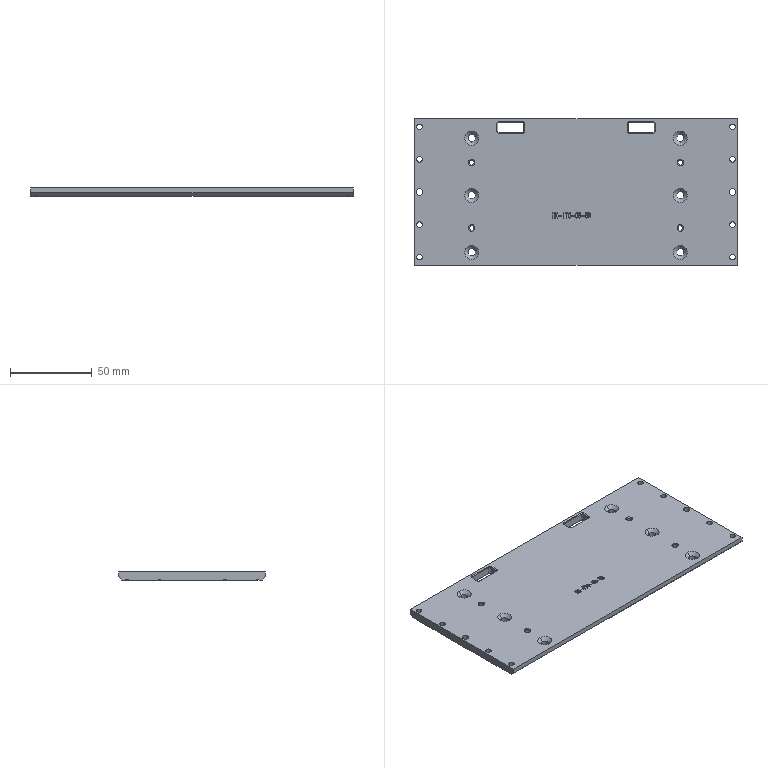NC program | NX | posted with a generic post | part box 198 x 90 x 5 mm
Lines 3242 to 4034 of 7160:
(ZLEVEL_PROFILE_COPY_1_COPY_COPY_COPY_1 , TOOL : D6A45)
N6422 T01 M6
N6424 G54
N6426 G17 G0 G90 X-98.522 Y18.565 S9500 M3
N6428 G43 Z30. H1
N6430 Z1.5
N6432 G94 G1 X-98.422 Y18.405 Z1.49 F1000.
N6434 X-98.29 Y18.203 Z1.477
N6436 X-97.857 Y17.759 Z1.445
N6438 X-97.339 Y17.416 Z1.412
N6440 X-96.76 Y17.19 Z1.38
N6442 X-96.147 Y17.093 Z1.347
N6444 X-95.527 Y17.128 Z1.315
N6446 X-94.929 Y17.293 Z1.282
N6448 X-94.379 Y17.582 Z1.25
N6450 X-94.002 Y17.882 Z1.224
N6452 X-93.599 Y18.354 Z1.192
N6454 X-93.304 Y18.901 Z1.159
N6456 X-93.132 Y19.497 Z1.127
N6458 X-93.091 Y20.117 Z1.094
N6460 X-93.182 Y20.731 Z1.062
N6462 X-93.401 Y21.312 Z1.029
N6464 X-93.738 Y21.833 Z0.997
N6466 X-94.071 Y22.181 Z0.971
N6468 X-94.578 Y22.54 Z0.939
N6470 X-95.149 Y22.784 Z0.906
N6472 X-95.758 Y22.901 Z0.874
N6474 X-96.379 Y22.886 Z0.841
N6476 X-96.982 Y22.74 Z0.809
N6478 X-97.541 Y22.469 Z0.776
N6480 X-98.03 Y22.086 Z0.744
N6482 X-98.188 Y21.904 Z0.731
N6484 X-98.237 Y21.848 Z0.727
N6486 X-98.619 Y21.317 Z0.693
N6488 X-98.657 Y21.245 Z0.689
N6490 X-98.76 Y21.024 Z0.676
N6492 X-98.918 Y20.378 Z0.641
N6494 X-98.927 Y19.713 Z0.606
N6496 X-98.788 Y19.062 Z0.571
N6498 X-98.692 Y18.838 Z0.558
N6500 X-98.422 Y18.405 Z0.532
N6502 X-98.29 Y18.203 Z0.519
N6504 X-97.857 Y17.759 Z0.486
N6506 X-97.339 Y17.416 Z0.454
N6508 X-96.76 Y17.19 Z0.421
N6510 X-96.147 Y17.093 Z0.389
N6512 X-95.527 Y17.128 Z0.356
N6514 X-94.929 Y17.293 Z0.324
N6516 X-94.379 Y17.582 Z0.291
N6518 X-94.002 Y17.882 Z0.266
N6520 X-93.599 Y18.354 Z0.233
N6522 X-93.304 Y18.901 Z0.201
N6524 X-93.132 Y19.497 Z0.168
N6526 X-93.091 Y20.117 Z0.136
N6528 X-93.182 Y20.731 Z0.103
N6530 X-93.401 Y21.312 Z0.071
N6532 X-93.738 Y21.833 Z0.038
N6534 X-94.071 Y22.181 Z0.013
N6536 X-94.578 Y22.54 Z-0.02
N6538 X-95.149 Y22.784 Z-0.052
N6540 X-95.758 Y22.901 Z-0.085
N6542 X-96.379 Y22.886 Z-0.117
N6544 X-96.982 Y22.74 Z-0.15
N6546 X-97.541 Y22.469 Z-0.182
N6548 X-98.03 Y22.086 Z-0.215
N6550 X-98.188 Y21.904 Z-0.227
N6552 X-98.237 Y21.848 Z-0.231
N6554 X-98.619 Y21.317 Z-0.266
N6556 X-98.657 Y21.245 Z-0.27
N6558 X-98.76 Y21.024 Z-0.283
N6560 X-98.918 Y20.378 Z-0.318
N6562 X-98.927 Y19.713 Z-0.352
N6564 X-98.788 Y19.062 Z-0.387
N6566 X-98.692 Y18.838 Z-0.4
N6568 X-98.422 Y18.405 F1300.
N6570 G3 X-98.188 Y21.904 R-2.901
N6572 G1 X-98.237 Y21.848
N6574 X-98.619 Y21.317
N6576 X-98.657 Y21.245
N6578 G3 X-98.692 Y18.838 R2.956
N6580 G1 X-98.624 Y18.722 Z-0.403
N6582 X-98.551 Y18.609 Z-0.406
N6584 X-98.413 Y18.411 Z-0.412
N6586 X-98.311 Y18.28 Z-0.416
N6588 X-98.207 Y18.149 Z-0.42
N6590 X-98.138 Y18.073 Z-0.422
N6592 X-97.983 Y17.922 Z-0.427
N6594 X-97.817 Y17.781 Z-0.432
N6596 X-97.642 Y17.655 Z-0.438
N6598 X-97.457 Y17.542 Z-0.443
N6600 X-97.266 Y17.444 Z-0.448
N6602 X-97.067 Y17.36 Z-0.453
N6604 X-96.864 Y17.292 Z-0.458
N6606 X-96.655 Y17.239 Z-0.463
N6608 X-96.445 Y17.202 Z-0.468
N6610 X-96.231 Y17.182 Z-0.473
N6612 X-96.019 Y17.177 Z-0.478
N6614 X-95.805 Y17.19 Z-0.483
N6616 X-95.595 Y17.216 Z-0.488
N6618 X-95.387 Y17.261 Z-0.493
N6620 X-95.183 Y17.318 Z-0.498
N6622 X-94.985 Y17.394 Z-0.503
N6624 X-94.793 Y17.48 Z-0.508
N6626 X-94.61 Y17.585 Z-0.513
N6628 X-94.433 Y17.698 Z-0.518
N6630 X-94.268 Y17.829 Z-0.523
N6632 X-94.163 Y17.924 Z-0.526
N6634 X-94.06 Y18.022 Z-0.53
N6636 X-93.969 Y18.121 Z-0.533
N6638 X-93.836 Y18.282 Z-0.538
N6640 X-93.717 Y18.454 Z-0.543
N6642 X-93.611 Y18.632 Z-0.548
N6644 X-93.519 Y18.819 Z-0.552
N6646 X-93.441 Y19.011 Z-0.557
N6648 X-93.379 Y19.209 Z-0.562
N6650 X-93.331 Y19.409 Z-0.567
N6652 X-93.3 Y19.613 Z-0.572
N6654 X-93.282 Y19.818 Z-0.577
N6656 X-93.281 Y20.024 Z-0.582
N6658 X-93.296 Y20.228 Z-0.586
N6660 X-93.326 Y20.431 Z-0.591
N6662 X-93.371 Y20.63 Z-0.596
N6664 X-93.43 Y20.826 Z-0.601
N6666 X-93.505 Y21.015 Z-0.606
N6668 X-93.592 Y21.199 Z-0.611
N6670 X-93.694 Y21.374 Z-0.615
N6672 X-93.807 Y21.542 Z-0.62
N6674 X-93.935 Y21.699 Z-0.625
N6676 X-94.071 Y21.848 Z-0.63
N6678 X-94.158 Y21.928 Z-0.632
N6680 X-94.245 Y22.007 Z-0.635
N6682 X-94.377 Y22.109 Z-0.639
N6684 X-94.544 Y22.22 Z-0.644
N6686 X-94.717 Y22.321 Z-0.649
N6688 X-94.899 Y22.405 Z-0.653
N6690 X-95.084 Y22.479 Z-0.658
N6692 X-95.276 Y22.534 Z-0.663
N6694 X-95.47 Y22.58 Z-0.667
N6696 X-95.666 Y22.605 Z-0.672
N6698 X-95.864 Y22.621 Z-0.677
N6700 X-96.062 Y22.616 Z-0.682
N6702 X-96.259 Y22.602 Z-0.686
N6704 X-96.453 Y22.567 Z-0.691
N6706 X-96.646 Y22.525 Z-0.695
N6708 X-96.831 Y22.461 Z-0.7
N6710 X-97.014 Y22.39 Z-0.705
N6712 X-97.188 Y22.299 Z-0.709
N6714 X-97.358 Y22.203 Z-0.714
N6716 X-97.514 Y22.087 Z-0.719
N6718 X-97.668 Y21.966 Z-0.723
N6720 X-97.805 Y21.828 Z-0.728
N6722 X-97.938 Y21.687 Z-0.732
N6724 X-97.98 Y21.636 Z-0.734
N6726 X-98.017 Y21.588 Z-0.735
N6728 X-98.052 Y21.539 Z-0.737
N6730 X-98.185 Y21.351 Z-0.742
N6732 X-98.311 Y21.151 Z-0.748
N6734 X-98.345 Y21.088 Z-0.749
N6736 X-98.408 Y20.924 Z-0.754
N6738 X-98.464 Y20.756 Z-0.758
N6740 X-98.522 Y20.473 Z-0.765
N6742 X-98.535 Y20.394 Z-0.766
N6744 X-98.547 Y20.216 Z-0.771
N6746 X-98.558 Y20.037 Z-0.775
N6748 X-98.529 Y19.682 Z-0.783
N6750 X-98.453 Y19.336 Z-0.792
N6752 X-98.396 Y19.169 Z-0.796
N6754 X-98.323 Y19.007 Z-0.8
N6756 X-98.231 Y18.848 Z-0.805
N6758 X-98.128 Y18.694 Z-0.81
N6760 X-97.9 Y18.407 Z-0.82
N6762 X-97.756 Y18.263 Z-0.826
N6764 X-97.605 Y18.126 Z-0.832
N6766 X-97.441 Y18.007 Z-0.837
N6768 X-97.27 Y17.898 Z-0.843
N6770 X-97.091 Y17.805 Z-0.848
N6772 X-96.903 Y17.729 Z-0.854
N6774 X-96.713 Y17.665 Z-0.86
N6776 X-96.516 Y17.622 Z-0.865
N6778 X-96.318 Y17.593 Z-0.871
N6780 X-96.118 Y17.581 Z-0.876
N6782 X-95.919 Y17.586 Z-0.882
N6784 X-95.721 Y17.606 Z-0.887
N6786 X-95.527 Y17.644 Z-0.893
N6788 X-95.334 Y17.693 Z-0.898
N6790 X-95.151 Y17.765 Z-0.904
N6792 X-94.968 Y17.841 Z-0.909
N6794 X-94.796 Y17.941 Z-0.915
N6796 X-94.635 Y18.05 Z-0.92
N6798 X-94.487 Y18.177 Z-0.926
N6800 X-94.343 Y18.31 Z-0.931
N6802 X-94.216 Y18.457 Z-0.936
N6804 X-94.097 Y18.611 Z-0.942
N6806 X-93.995 Y18.776 Z-0.947
N6808 X-93.904 Y18.947 Z-0.952
N6810 X-93.829 Y19.124 Z-0.958
N6812 X-93.77 Y19.308 Z-0.963
N6814 X-93.725 Y19.495 Z-0.969
N6816 X-93.697 Y19.685 Z-0.974
N6818 X-93.685 Y19.875 Z-0.979
N6820 X-93.687 Y20.067 Z-0.984
N6822 X-93.708 Y20.255 Z-0.99
N6824 X-93.739 Y20.443 Z-0.995
N6826 X-93.766 Y20.546 Z-0.998
N6828 X-93.795 Y20.649 Z-1.001
N6830 X-93.852 Y20.804 Z-1.005
N6832 X-93.934 Y20.974 Z-1.011
N6834 X-94.02 Y21.142 Z-1.016
N6836 X-94.124 Y21.292 Z-1.021
N6838 X-94.243 Y21.443 Z-1.026
N6840 X-94.375 Y21.575 Z-1.032
N6842 X-94.51 Y21.703 Z-1.037
N6844 X-94.66 Y21.813 Z-1.042
N6846 X-94.815 Y21.916 Z-1.047
N6848 X-94.979 Y22. Z-1.052
N6850 X-95.149 Y22.075 Z-1.057
N6852 X-95.323 Y22.132 Z-1.062
N6854 X-95.502 Y22.176 Z-1.067
N6856 X-95.683 Y22.204 Z-1.073
N6858 X-95.866 Y22.218 Z-1.078
N6860 X-96.048 Y22.214 Z-1.083
N6862 X-96.23 Y22.2 Z-1.088
N6864 X-96.408 Y22.165 Z-1.093
N6866 X-96.585 Y22.123 Z-1.098
N6868 X-96.754 Y22.059 Z-1.103
N6870 X-96.921 Y21.99 Z-1.108
N6872 X-97.087 Y21.897 Z-1.113
N6874 X-97.229 Y21.805 Z-1.118
N6876 X-97.365 Y21.689 Z-1.123
N6878 X-97.501 Y21.571 Z-1.128
N6880 X-97.548 Y21.522 Z-1.13
N6882 X-97.737 Y21.293 Z-1.138
N6884 X-97.928 Y21.005 Z-1.147
N6886 X-97.977 Y20.919 Z-1.15
N6888 X-98.021 Y20.83 Z-1.153
N6890 X-98.056 Y20.726 Z-1.156
N6892 X-98.13 Y20.402 Z-1.165
N6894 X-98.143 Y20.242 Z-1.17
N6896 X-98.156 Y20.083 Z-1.174
N6898 X-98.147 Y19.924 Z-1.178
N6900 X-98.136 Y19.765 Z-1.183
N6902 X-98.101 Y19.574 Z-1.188
N6904 X-98.063 Y19.428 Z-1.192
N6906 X-98.017 Y19.299 Z-1.196
N6908 X-97.957 Y19.177 Z-1.2
N6910 X-97.953 Y19.142 Z-1.201
N6912 X-97.935 Y19.114 Z-1.202
N6914 X-97.742 Y18.842 Z-1.213
N6916 X-97.615 Y18.69 Z-1.22
N6918 X-97.48 Y18.545 Z-1.227
N6920 X-97.38 Y18.455 Z-1.231
N6922 X-97.274 Y18.376 Z-1.235
N6924 X-97.169 Y18.302 Z-1.24
N6926 X-96.972 Y18.195 Z-1.247
N6928 X-96.898 Y18.157 Z-1.25
N6930 X-96.82 Y18.126 Z-1.253
N6932 X-96.636 Y18.063 Z-1.259
N6934 X-96.447 Y18.016 Z-1.266
N6936 X-96.31 Y17.99 Z-1.271
N6938 X-96.183 Y17.983 Z-1.275
N6940 X-96.067 Y17.98 Z-1.279
N6942 X-95.906 Y17.986 Z-1.284
N6944 X-95.78 Y18. Z-1.288
N6946 X-95.688 Y18.014 Z-1.291
N6948 X-95.506 Y18.065 Z-1.298
N6950 X-95.326 Y18.123 Z-1.304
N6952 X-95.201 Y18.175 Z-1.309
N6954 X-95.139 Y18.201 Z-1.311
N6956 X-95.09 Y18.231 Z-1.313
N6958 X-94.991 Y18.294 Z-1.317
N6960 X-94.84 Y18.403 Z-1.323
N6962 X-94.697 Y18.523 Z-1.329
N6964 X-94.572 Y18.66 Z-1.335
N6966 X-94.452 Y18.801 Z-1.342
N6968 X-94.367 Y18.931 Z-1.347
N6970 X-94.314 Y19.023 Z-1.35
N6972 X-94.267 Y19.12 Z-1.354
N6974 X-94.196 Y19.288 Z-1.36
N6976 X-94.144 Y19.464 Z-1.366
N6978 X-94.11 Y19.606 Z-1.371
N6980 X-94.096 Y19.726 Z-1.375
N6982 X-94.087 Y19.824 Z-1.379
N6984 X-94.084 Y19.969 Z-1.383
N6986 X-94.088 Y20.089 Z-1.387
N6988 X-94.101 Y20.185 Z-1.391
N6990 X-94.135 Y20.361 Z-1.397
N6992 X-94.182 Y20.535 Z-1.403
N6994 X-94.223 Y20.658 Z-1.407
N6996 X-94.248 Y20.718 Z-1.409
N6998 X-94.273 Y20.766 Z-1.411
N7000 X-94.326 Y20.862 Z-1.415
N7002 X-94.421 Y21.011 Z-1.421
N7004 X-94.524 Y21.155 Z-1.427
N7006 X-94.648 Y21.281 Z-1.433
N7008 X-94.777 Y21.402 Z-1.439
N7010 X-94.856 Y21.462 Z-1.442
N7012 X-94.959 Y21.534 Z-1.446
N7014 X-95.068 Y21.596 Z-1.45
N7016 X-95.225 Y21.671 Z-1.456
N7018 X-95.389 Y21.732 Z-1.462
N7020 X-95.593 Y21.785 Z-1.469
N7022 X-95.726 Y21.808 Z-1.474
N7024 X-95.908 Y21.818 Z-1.48
N7026 X-96.07 Y21.813 Z-1.485
N7028 X-96.203 Y21.8 Z-1.49
N7030 X-96.27 Y21.792 Z-1.492
N7032 X-96.316 Y21.78 Z-1.493
N7034 X-96.406 Y21.756 Z-1.497
N7036 X-96.567 Y21.703 Z-1.502
N7038 X-96.724 Y21.639 Z-1.508
N7040 X-96.893 Y21.545 Z-1.514
N7042 X-97.014 Y21.466 Z-1.519
N7044 X-97.14 Y21.355 Z-1.525
N7046 X-97.262 Y21.24 Z-1.531
N7048 X-97.295 Y21.203 Z-1.532
N7050 X-97.393 Y21.083 Z-1.537
N7052 X-97.485 Y20.958 Z-1.543
N7054 X-97.573 Y20.821 Z-1.548
N7056 X-97.633 Y20.722 Z-1.552
N7058 X-97.659 Y20.659 Z-1.554
N7060 X-97.703 Y20.509 Z-1.559
N7062 X-97.738 Y20.331 Z-1.565
N7064 X-97.757 Y20.061 Z-1.575
N7066 X-97.737 Y19.793 Z-1.584
N7068 X-97.678 Y19.532 Z-1.593
N7070 X-97.639 Y19.427 Z-1.596
N7072 X-97.599 Y19.322 Z-1.6
N7074 X-97.584 Y19.289 Z-1.602
N7076 X-97.49 Y19.165 Z-1.608
N7078 X-97.358 Y18.994 Z-1.617
N7080 X-97.262 Y18.895 Z-1.623
N7082 X-97.175 Y18.809 Z-1.628
N7084 X-97.092 Y18.741 Z-1.633
N7086 X-96.961 Y18.642 Z-1.64
N7088 X-96.891 Y18.601 Z-1.643
N7090 X-96.785 Y18.545 Z-1.648
N7092 X-96.622 Y18.482 Z-1.656
N7094 X-96.456 Y18.427 Z-1.663
N7096 X-96.425 Y18.42 Z-1.664
N7098 X-96.27 Y18.395 Z-1.671
N7100 X-96.114 Y18.381 Z-1.678
N7102 X-95.984 Y18.379 Z-1.683
N7104 X-95.87 Y18.393 Z-1.688
N7106 X-95.772 Y18.407 Z-1.692
N7108 X-95.643 Y18.438 Z-1.698
N7110 X-95.533 Y18.468 Z-1.703
N7112 X-95.447 Y18.505 Z-1.707
N7114 X-95.296 Y18.579 Z-1.714
N7116 X-95.153 Y18.667 Z-1.721
N7118 X-95.053 Y18.742 Z-1.726
N7120 X-94.969 Y18.815 Z-1.731
N7122 X-94.901 Y18.886 Z-1.735
N7124 X-94.808 Y18.993 Z-1.741
N7126 X-94.766 Y19.049 Z-1.744
N7128 X-94.703 Y19.15 Z-1.749
N7130 X-94.636 Y19.273 Z-1.755
N7132 X-94.592 Y19.373 Z-1.76
N7134 X-94.565 Y19.447 Z-1.763
N7136 X-94.529 Y19.573 Z-1.769
N7138 X-94.512 Y19.637 Z-1.772
N7140 X-94.504 Y19.679 Z-1.774
N7142 X-94.496 Y19.764 Z-1.777
N7144 X-94.483 Y19.914 Z-1.784
N7146 X-94.487 Y20.021 Z-1.788
N7148 X-94.493 Y20.085 Z-1.791
N7150 X-94.512 Y20.218 Z-1.797
N7152 X-94.532 Y20.322 Z-1.801
N7154 X-94.56 Y20.397 Z-1.805
N7156 X-94.615 Y20.545 Z-1.811
N7158 X-94.688 Y20.686 Z-1.818
N7160 X-94.753 Y20.794 Z-1.823
N7162 X-94.815 Y20.878 Z-1.828
N7164 X-94.871 Y20.94 Z-1.831
N7166 X-94.983 Y21.047 Z-1.838
N7168 X-95.104 Y21.145 Z-1.845
N7170 X-95.196 Y21.212 Z-1.85
N7172 X-95.287 Y21.26 Z-1.854
N7174 X-95.37 Y21.3 Z-1.858
N7176 X-95.41 Y21.314 Z-1.86
N7178 X-95.535 Y21.355 Z-1.865
N7180 X-95.662 Y21.387 Z-1.871
N7182 X-95.78 Y21.412 Z-1.876
N7184 X-95.88 Y21.417 Z-1.88
N7186 X-95.963 Y21.416 Z-1.884
N7188 X-96.091 Y21.41 Z-1.889
N7190 X-96.19 Y21.398 Z-1.893
N7192 X-96.26 Y21.379 Z-1.896
N7194 X-96.402 Y21.338 Z-1.903
N7196 X-96.54 Y21.281 Z-1.909
N7198 X-96.643 Y21.231 Z-1.914
N7200 X-96.726 Y21.179 Z-1.918
N7202 X-96.792 Y21.13 Z-1.922
N7204 X-96.901 Y21.033 Z-1.928
N7206 X-97.005 Y20.93 Z-1.934
N7208 X-97.068 Y20.851 Z-1.938
N7210 X-97.17 Y20.714 Z-1.946
N7212 X-97.23 Y20.62 Z-1.95
N7214 X-97.273 Y20.548 Z-1.954
N7216 X-97.29 Y20.496 Z-1.956
N7218 X-97.319 Y20.373 Z-1.962
N7220 X-97.347 Y20.25 Z-1.967
N7222 X-97.358 Y20.117 Z-1.973
N7224 X-97.359 Y19.99 Z-1.978
N7226 X-97.343 Y19.858 Z-1.984
N7228 X-97.322 Y19.734 Z-1.989
N7230 X-97.288 Y19.62 Z-1.994
N7232 X-97.263 Y19.552 Z-1.997
N7234 X-97.249 Y19.522 Z-1.999
N7236 X-97.228 Y19.494 Z-2.
N7238 G3 X-96.338 Y18.744 R1.379
N7240 X-94.717 Y19.776 R1.3
N7242 X-97.022 Y20.812 R1.306
N7244 X-97.254 Y19.555 R1.185
N7246 G1 X-97.228 Y19.494
N7248 Z-0.5
N7250 G0 Z30.
N7252 X-97.495 Y42.494
N7254 Z1.5
N7256 G1 X-97.645 Y42.398 Z1.491 F1000.
N7258 X-98.004 Y42.094 Z1.466
N7260 X-98.323 Y41.749 Z1.441
N7262 X-98.482 Y41.523 Z1.427
N7264 X-98.575 Y41.386 Z1.418
N7266 X-98.674 Y41.24 Z1.409
N7268 X-98.771 Y41.016 Z1.396
N7270 X-98.809 Y40.844 Z1.387
N7272 X-98.91 Y40.404 Z1.363
N7274 X-98.936 Y39.82 Z1.333
N7276 X-98.846 Y39.243 Z1.302
N7278 X-98.766 Y39.015 Z1.289
N7280 X-98.69 Y38.814 Z1.278
N7282 X-98.55 Y38.567 Z1.263
N7284 X-98.417 Y38.399 Z1.252
N7286 X-98.284 Y38.198 Z1.239
N7288 X-97.839 Y37.746 Z1.206
N7290 X-97.307 Y37.401 Z1.173
N7292 X-96.713 Y37.179 Z1.14
N7294 X-96.085 Y37.091 Z1.106
N7296 X-95.453 Y37.141 Z1.073
N7298 X-94.847 Y37.327 Z1.04
N7300 X-94.296 Y37.64 Z1.007
N7302 X-93.929 Y37.953 Z0.982
N7304 X-93.535 Y38.45 Z0.948
N7306 X-93.258 Y39.021 Z0.915
N7308 X-93.111 Y39.638 Z0.882
N7310 X-93.102 Y40.272 Z0.849
N7312 X-93.229 Y40.893 Z0.815
N7314 X-93.489 Y41.471 Z0.782
N7316 X-93.867 Y41.98 Z0.749
N7318 X-94.045 Y42.142 Z0.736
N7320 X-94.217 Y42.308 Z0.724
N7322 X-94.697 Y42.625 Z0.694
N7324 X-95.232 Y42.838 Z0.663
N7326 X-95.798 Y42.94 Z0.633
N7328 X-96.374 Y42.925 Z0.603
N7330 X-96.934 Y42.795 Z0.573
N7332 X-97.152 Y42.699 Z0.56
N7334 X-97.375 Y42.57 Z0.547
N7336 X-97.412 Y42.547 Z0.545
N7338 X-97.645 Y42.398 Z0.53
N7340 X-98.004 Y42.094 Z0.506
N7342 X-98.323 Y41.749 Z0.481
N7344 X-98.482 Y41.523 Z0.466
N7346 X-98.575 Y41.386 Z0.458
N7348 X-98.674 Y41.24 Z0.449
N7350 X-98.771 Y41.016 Z0.436
N7352 X-98.809 Y40.844 Z0.426
N7354 X-98.91 Y40.404 Z0.403
N7356 X-98.936 Y39.82 Z0.372
N7358 X-98.846 Y39.243 Z0.342
N7360 X-98.766 Y39.015 Z0.329
N7362 X-98.69 Y38.814 Z0.318
N7364 X-98.55 Y38.567 Z0.303
N7366 X-98.417 Y38.399 Z0.292
N7368 X-98.284 Y38.198 Z0.279
N7370 X-97.839 Y37.746 Z0.246
N7372 X-97.307 Y37.401 Z0.212
N7374 X-96.713 Y37.179 Z0.179
N7376 X-96.085 Y37.091 Z0.146
N7378 X-95.453 Y37.141 Z0.113
N7380 X-94.847 Y37.327 Z0.08
N7382 X-94.296 Y37.64 Z0.046
N7384 X-93.929 Y37.953 Z0.021
N7386 X-93.535 Y38.45 Z-0.012
N7388 X-93.258 Y39.021 Z-0.045
N7390 X-93.111 Y39.638 Z-0.079
N7392 X-93.102 Y40.272 Z-0.112
N7394 X-93.229 Y40.893 Z-0.145
N7396 X-93.489 Y41.471 Z-0.178
N7398 X-93.867 Y41.98 Z-0.212
N7400 X-94.045 Y42.142 Z-0.224
N7402 X-94.217 Y42.308 Z-0.237
N7404 X-94.697 Y42.625 Z-0.267
N7406 X-95.232 Y42.838 Z-0.297
N7408 X-95.798 Y42.94 Z-0.327
N7410 X-96.374 Y42.925 Z-0.357
N7412 X-96.934 Y42.795 Z-0.388
N7414 X-97.152 Y42.699 Z-0.4
N7416 X-97.375 Y42.57 F1300.
N7418 X-97.412 Y42.547
N7420 G3 X-98.482 Y41.523 R3.818
N7422 G1 X-98.575 Y41.386
N7424 G3 X-98.809 Y40.844 R1.559
N7426 G1 X-98.856 Y40.64
N7428 G3 X-98.766 Y39.015 R2.926
N7430 X-98.417 Y38.399 R2.289
N7432 X-94.045 Y42.142 R-2.9
N7434 X-97.152 Y42.699 R2.832
N7436 G1 X-97.262 Y42.632 Z-0.403
N7438 X-97.408 Y42.541 Z-0.407
N7440 X-97.611 Y42.4 Z-0.413
N7442 X-97.802 Y42.242 Z-0.419
N7444 X-97.897 Y42.162 Z-0.422
N7446 X-98.028 Y42.031 Z-0.426
N7448 X-98.152 Y41.893 Z-0.43
N7450 X-98.305 Y41.701 Z-0.436
N7452 X-98.447 Y41.501 Z-0.442
N7454 X-98.534 Y41.363 Z-0.446
N7456 X-98.606 Y41.236 Z-0.449
N7458 X-98.667 Y41.104 Z-0.453
N7460 X-98.751 Y40.826 Z-0.459
N7462 X-98.795 Y40.626 Z-0.464
N7464 X-98.827 Y40.427 Z-0.469
N7466 X-98.847 Y40.227 Z-0.474
N7468 X-98.849 Y40.026 Z-0.478
N7470 X-98.844 Y39.826 Z-0.483
N7472 X-98.813 Y39.628 Z-0.488
N7474 X-98.782 Y39.431 Z-0.493
N7476 X-98.726 Y39.24 Z-0.497
N7478 X-98.669 Y39.05 Z-0.502
N7480 X-98.618 Y38.923 Z-0.505
N7482 X-98.554 Y38.802 Z-0.508
N7484 X-98.521 Y38.748 Z-0.51
N7486 X-98.324 Y38.467 Z-0.518
N7488 X-98.192 Y38.296 Z-0.523
N7490 X-98.048 Y38.135 Z-0.528
N7492 X-97.896 Y37.984 Z-0.533
N7494 X-97.729 Y37.848 Z-0.538
N7496 X-97.653 Y37.791 Z-0.54
N7498 X-97.517 Y37.7 Z-0.544
N7500 X-97.376 Y37.617 Z-0.548
N7502 X-97.187 Y37.521 Z-0.553
N7504 X-96.99 Y37.443 Z-0.558
N7506 X-96.79 Y37.379 Z-0.563
N7508 X-96.584 Y37.331 Z-0.568
N7510 X-96.377 Y37.299 Z-0.573
N7512 X-96.167 Y37.283 Z-0.578
N7514 X-95.958 Y37.284 Z-0.583
N7516 X-95.749 Y37.299 Z-0.588
N7518 X-95.544 Y37.333 Z-0.593
N7520 X-95.34 Y37.379 Z-0.598
N7522 X-95.144 Y37.444 Z-0.602
N7524 X-94.95 Y37.52 Z-0.607
N7526 X-94.767 Y37.615 Z-0.612
N7528 X-94.587 Y37.718 Z-0.617
N7530 X-94.421 Y37.841 Z-0.622
N7532 X-94.26 Y37.969 Z-0.627
N7534 X-94.117 Y38.116 Z-0.632
N7536 X-93.977 Y38.266 Z-0.636
N7538 X-93.914 Y38.345 Z-0.639
N7540 X-93.743 Y38.602 Z-0.646
N7542 X-93.652 Y38.785 Z-0.651
N7544 X-93.564 Y38.969 Z-0.656
N7546 X-93.503 Y39.162 Z-0.661
N7548 X-93.444 Y39.357 Z-0.665
N7550 X-93.414 Y39.557 Z-0.67
N7552 X-93.385 Y39.757 Z-0.675
N7554 Y39.959 Z-0.68
N7556 X-93.389 Y40.16 Z-0.684
N7558 X-93.42 Y40.359 Z-0.689
N7560 X-93.453 Y40.557 Z-0.694
N7562 X-93.514 Y40.747 Z-0.699
N7564 X-93.577 Y40.938 Z-0.703
N7566 X-93.757 Y41.294 Z-0.713
N7568 X-93.99 Y41.616 Z-0.722
N7570 X-94.128 Y41.758 Z-0.727
N7572 X-94.268 Y41.898 Z-0.731
N7574 X-94.346 Y41.963 Z-0.734
N7576 X-94.568 Y42.132 Z-0.74
N7578 X-94.881 Y42.323 Z-0.749
N7580 X-94.978 Y42.373 Z-0.751
N7582 X-95.029 Y42.393 Z-0.753
N7584 X-95.093 Y42.414 Z-0.754
N7586 X-95.223 Y42.453 Z-0.758
N7588 X-95.4 Y42.494 Z-0.762
N7590 X-95.578 Y42.532 Z-0.766
N7592 X-95.759 Y42.544 Z-0.77
N7594 X-95.94 Y42.557 Z-0.775
N7596 X-96.119 Y42.544 Z-0.779
N7598 X-96.299 Y42.531 Z-0.783
N7600 X-96.65 Y42.456 Z-0.792
N7602 X-96.818 Y42.396 Z-0.796
N7604 X-96.983 Y42.326 Z-0.8
N7606 X-97.155 Y42.224 Z-0.806
N7608 X-97.324 Y42.119 Z-0.811
N7610 X-97.63 Y41.864 Z-0.822
N7612 X-97.769 Y41.719 Z-0.828
N7614 X-97.906 Y41.573 Z-0.833
N7616 X-98.136 Y41.244 Z-0.844
N7618 X-98.21 Y41.117 Z-0.848
N7620 X-98.28 Y40.988 Z-0.852
N7622 X-98.297 Y40.94 Z-0.854
N7624 X-98.314 Y40.892 Z-0.855
N7626 X-98.366 Y40.7 Z-0.861
N7628 X-98.412 Y40.508 Z-0.866
N7630 X-98.435 Y40.312 Z-0.872
N7632 X-98.453 Y40.116 Z-0.877
N7634 X-98.442 Y39.92 Z-0.882
N7636 X-98.429 Y39.724 Z-0.888
N7638 X-98.389 Y39.519 Z-0.894
N7640 X-98.345 Y39.343 Z-0.899
N7642 X-98.295 Y39.19 Z-0.903
N7644 X-98.25 Y39.07 Z-0.907
N7646 X-98.201 Y38.986 Z-0.909
N7648 X-97.974 Y38.664 Z-0.92
N7650 X-97.849 Y38.511 Z-0.926
N7652 X-97.711 Y38.368 Z-0.931
N7654 X-97.566 Y38.234 Z-0.937
N7656 X-97.41 Y38.113 Z-0.942
N7658 X-97.352 Y38.072 Z-0.944
N7660 X-97.292 Y38.033 Z-0.946
N7662 X-97.064 Y37.91 Z-0.953
N7664 X-96.849 Y37.82 Z-0.96
N7666 X-96.69 Y37.767 Z-0.964
N7668 X-96.494 Y37.728 Z-0.97
N7670 X-96.297 Y37.695 Z-0.975
N7672 X-96.157 Y37.685 Z-0.979
N7674 X-96.025 Y37.679 Z-0.983
N7676 X-95.9 Y37.689 Z-0.986
N7678 X-95.704 Y37.713 Z-0.992
N7680 X-95.51 Y37.751 Z-0.997
N7682 X-95.321 Y37.805 Z-1.003
N7684 X-95.137 Y37.877 Z-1.008
N7686 X-94.963 Y37.965 Z-1.014
N7688 X-94.794 Y38.065 Z-1.019
N7690 X-94.639 Y38.182 Z-1.025
N7692 X-94.489 Y38.307 Z-1.03
N7694 X-94.343 Y38.459 Z-1.036
N7696 X-94.23 Y38.595 Z-1.041
N7698 X-94.127 Y38.758 Z-1.046
N7700 X-94.027 Y38.923 Z-1.051
N7702 X-93.97 Y39.044 Z-1.055
N7704 X-93.918 Y39.161 Z-1.059
N7706 X-93.882 Y39.279 Z-1.062
N7708 X-93.835 Y39.464 Z-1.067
N7710 X-93.801 Y39.652 Z-1.073
N7712 X-93.784 Y39.842 Z-1.078
N7714 X-93.785 Y40.032 Z-1.083
N7716 X-93.803 Y40.22 Z-1.088
N7718 X-93.834 Y40.407 Z-1.094
N7720 X-93.884 Y40.589 Z-1.099
N7722 X-93.944 Y40.767 Z-1.104
N7724 X-94.032 Y40.958 Z-1.11
N7726 X-94.112 Y41.102 Z-1.114
N7728 X-94.222 Y41.253 Z-1.12
N7730 X-94.338 Y41.4 Z-1.125
N7732 X-94.523 Y41.588 Z-1.132
N7734 X-94.615 Y41.664 Z-1.135
N7736 X-94.892 Y41.863 Z-1.145
N7738 X-95.011 Y41.935 Z-1.149
N7740 X-95.108 Y41.995 Z-1.152
N7742 X-95.192 Y42.022 Z-1.154
N7744 X-95.354 Y42.071 Z-1.159
N7746 X-95.519 Y42.112 Z-1.164
N7748 X-95.685 Y42.136 Z-1.168
N7750 X-95.852 Y42.156 Z-1.173
N7752 X-96.019 Y42.15 Z-1.178
N7754 X-96.187 Y42.143 Z-1.182
N7756 X-96.514 Y42.08 Z-1.191
N7758 X-96.661 Y42.028 Z-1.196
N7760 X-96.807 Y41.976 Z-1.2
N7762 X-96.978 Y41.864 Z-1.207
N7764 X-97.148 Y41.749 Z-1.214
N7766 X-97.301 Y41.615 Z-1.22
N7768 X-97.452 Y41.478 Z-1.227
N7770 X-97.582 Y41.323 Z-1.234
N7772 X-97.707 Y41.163 Z-1.241
N7774 X-97.809 Y41.007 Z-1.247
N7776 X-97.86 Y40.928 Z-1.25
N7778 X-97.88 Y40.893 Z-1.252
N7780 X-97.916 Y40.821 Z-1.254
N7782 X-97.966 Y40.67 Z-1.26
N7784 X-98.009 Y40.491 Z-1.266
N7786 X-98.031 Y40.321 Z-1.271
N7788 X-98.05 Y40.15 Z-1.277
N7790 X-98.049 Y39.973 Z-1.283
N7792 X-98.034 Y39.808 Z-1.289
N7794 X-98.001 Y39.642 Z-1.294
N7796 X-97.964 Y39.476 Z-1.3
N7798 X-97.923 Y39.343 Z-1.305
N7800 X-97.885 Y39.24 Z-1.308
N7802 X-97.845 Y39.168 Z-1.311
N7804 X-97.625 Y38.865 Z-1.324
N7806 X-97.499 Y38.727 Z-1.33
N7808 X-97.369 Y38.593 Z-1.336
N7810 X-97.223 Y38.478 Z-1.342
N7812 X-97.072 Y38.369 Z-1.349
N7814 X-96.979 Y38.32 Z-1.352
N7816 X-96.865 Y38.261 Z-1.356
N7818 X-96.745 Y38.213 Z-1.361
N7820 X-96.576 Y38.155 Z-1.367
N7822 X-96.4 Y38.118 Z-1.373
N7824 X-96.223 Y38.095 Z-1.379
N7826 X-96.045 Y38.086 Z-1.385
N7828 X-95.848 Y38.098 Z-1.391
N7830 X-95.692 Y38.121 Z-1.397
N7832 X-95.567 Y38.152 Z-1.401
N7834 X-95.453 Y38.182 Z-1.405
N7836 X-95.355 Y38.223 Z-1.408
N7838 X-95.196 Y38.295 Z-1.414
N7840 X-95.044 Y38.382 Z-1.42
N7842 X-94.935 Y38.451 Z-1.425
N7844 X-94.847 Y38.527 Z-1.428
N7846 X-94.769 Y38.594 Z-1.432
N7848 X-94.663 Y38.711 Z-1.437
N7850 X-94.558 Y38.828 Z-1.442
N7852 X-94.539 Y38.853 Z-1.444
N7854 X-94.449 Y38.999 Z-1.449
N7856 X-94.363 Y39.147 Z-1.455
N7858 X-94.293 Y39.309 Z-1.461
N7860 X-94.276 Y39.361 Z-1.463
N7862 X-94.244 Y39.468 Z-1.467
N7864 X-94.212 Y39.634 Z-1.472
N7866 X-94.188 Y39.802 Z-1.478
N7868 X-94.185 Y39.987 Z-1.484
N7870 X-94.193 Y40.14 Z-1.489
N7872 X-94.224 Y40.318 Z-1.495
N7874 X-94.263 Y40.467 Z-1.501
N7876 X-94.303 Y40.587 Z-1.505
N7878 X-94.324 Y40.647 Z-1.507
N7880 X-94.345 Y40.69 Z-1.508
N7882 X-94.39 Y40.775 Z-1.512
N7884 X-94.474 Y40.918 Z-1.517
N7886 X-94.57 Y41.053 Z-1.523
N7888 X-94.624 Y41.118 Z-1.526
N7890 X-94.682 Y41.18 Z-1.528
N7892 X-94.803 Y41.302 Z-1.534
N7894 X-95.071 Y41.506 Z-1.546
N7896 X-95.185 Y41.57 Z-1.55
N7898 X-95.281 Y41.628 Z-1.554
N7900 X-95.369 Y41.66 Z-1.557
N7902 X-95.529 Y41.703 Z-1.562
N7904 X-95.692 Y41.737 Z-1.568
N7906 X-95.879 Y41.755 Z-1.574
N7908 X-96.021 Y41.756 Z-1.579
N7910 X-96.199 Y41.736 Z-1.585
N7912 X-96.345 Y41.711 Z-1.59
N7914 X-96.49 Y41.664 Z-1.595
N7916 X-96.635 Y41.616 Z-1.6
N7918 X-96.777 Y41.522 Z-1.607
N7920 X-96.918 Y41.424 Z-1.614
N7922 X-97.169 Y41.195 Z-1.629
N7924 X-97.264 Y41.086 Z-1.635
N7926 X-97.31 Y41.026 Z-1.638
N7928 X-97.381 Y40.933 Z-1.643
N7930 X-97.476 Y40.782 Z-1.651
N7932 X-97.534 Y40.688 Z-1.655
N7934 X-97.552 Y40.648 Z-1.657
N7936 X-97.587 Y40.542 Z-1.662
N7938 X-97.611 Y40.432 Z-1.667
N7940 X-97.631 Y40.32 Z-1.671
N7942 X-97.645 Y40.185 Z-1.677
N7944 X-97.65 Y40.117 Z-1.68
N7946 Y40.073 Z-1.682
N7948 X-97.649 Y39.987 Z-1.686
N7950 X-97.636 Y39.855 Z-1.691
N7952 X-97.618 Y39.746 Z-1.696
N7954 X-97.6 Y39.66 Z-1.7
N7956 X-97.557 Y39.52 Z-1.706
N7958 X-97.521 Y39.417 Z-1.71
N7960 X-97.489 Y39.353 Z-1.713
N7962 X-97.29 Y39.087 Z-1.728
N7964 X-97.139 Y38.93 Z-1.737
N7966 X-97.052 Y38.848 Z-1.742
N7968 X-96.959 Y38.777 Z-1.747
N7970 X-96.87 Y38.713 Z-1.752
N7972 X-96.776 Y38.667 Z-1.756
N7974 X-96.635 Y38.602 Z-1.763
N7976 X-96.488 Y38.548 Z-1.769
N7978 X-96.379 Y38.52 Z-1.774
N7980 X-96.277 Y38.501 Z-1.778
N7982 X-96.184 Y38.493 Z-1.782
N7984 X-96.032 Y38.49 Z-1.789
N7986 X-95.879 Y38.5 Z-1.795
N7988 X-95.766 Y38.513 Z-1.8
N7990 X-95.669 Y38.54 Z-1.804
N7992 X-95.583 Y38.566 Z-1.808
N7994 X-95.47 Y38.61 Z-1.813
N7996 X-95.378 Y38.65 Z-1.818
N7998 X-95.31 Y38.689 Z-1.821
N8000 X-95.187 Y38.773 Z-1.827